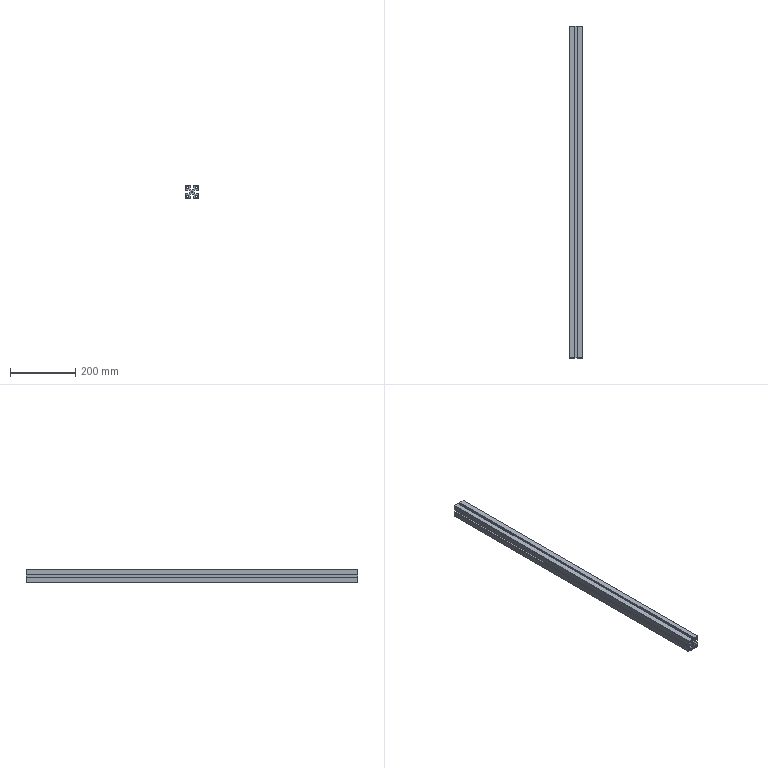Part | STEP file | 01-05 Bracket crossbar 3 | 1 solid | 68 faces | box 40 x 1020 x 40 mm | volume 938165 mm3 | plane 54 | cylinder 14 | commonest cylinder face diameters 6 x10 2 x4